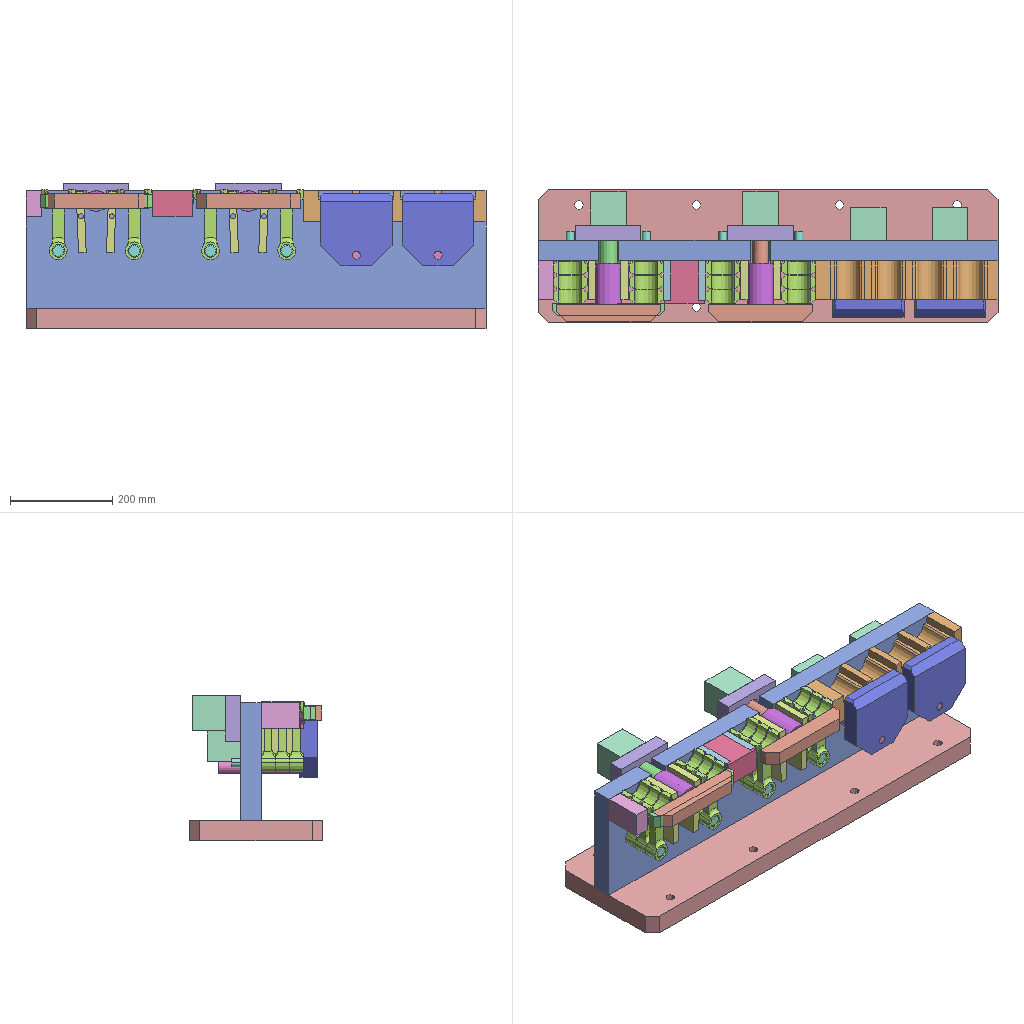Assembly | SolidWorks | 20 different items | 48 placed | box 900 x 260 x 285 mm
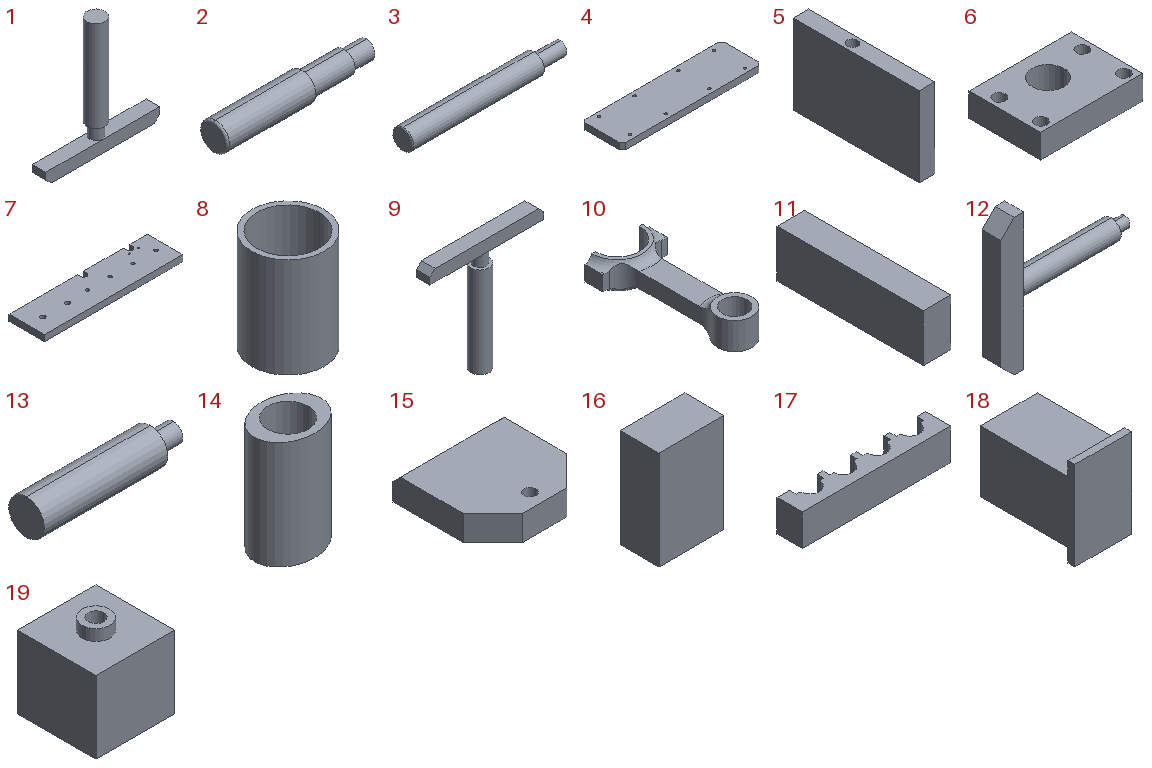Parts list (item | name | quantity | parent item | size | volume | features):
1 | (subassembly) | x1 | - | 220 x 35 x 223 mm | 309149 mm3 | features AEMSimFeature 1
2 | - | x4 | - | 138 x 25 x 25 mm | 55164 mm3 | features Fillet 1, Revolution 1
3 | - | x2 | - | 192 x 25 x 25 mm | 84936 mm3 | features Chamfer 1, Revolution 1
4 | - | x1 | - | 900 x 260 x 40 mm | 9255366 mm3 | features Chamfer 1, Extrusion 1, HoleWzd 1
5 | - | x4 | - | 15 x 120 x 76 mm | 130831 mm3 | features Extrusion 1, ICE 1
6 | - | x2 | - | 128 x 90 x 30 mm | 286695 mm3 | features Extrusion 1, HoleWzd 1, ICE 1
7 | - | x1 | - | 900 x 230 x 40 mm | 8056344 mm3 | features ICE 4, LPattern 2, Extrusion 1
8 | - | x2 | - | 29 x 29 x 40 mm | 6786 mm3 | features Extrusion 1
9 | - | x1 | in 1 | 220 x 35 x 223 mm | 309149 mm3 | features ICE 2, Chamfer 1, Extrusion 1
10 | - | x12 | - | 66 x 137 x 27.5 mm | 56707 mm3 | features Fillet 4, ICE 3, Extrusion 1, MirrorPattern 1
11 | - | x2 | - | 14.5 x 77 x 25 mm | 27913 mm3 | features Extrusion 1
12 | - | x2 | - | 199 x 30 x 204 mm | 289524 mm3 | features Chamfer 1, ICE 1, Revolution 1
13 | - | x2 | - | 125 x 30 x 30 mm | 78241 mm3 | features Revolution 1
14 | - | x2 | - | 50 x 40 x 80 mm | 69122 mm3 | features Extrusion 1, ICE 1
15 | - | x2 | - | 140 x 140 x 34 mm | 588897 mm3 | features Chamfer 3, Extrusion 1, ICE 1
16 | - | x1 | - | 50 x 30 x 76 mm | 114000 mm3 | features Extrusion 1
17 | - | x1 | - | 357 x 60 x 76 mm | 1051674 mm3 | features ICE 2, Extrusion 1, Fillet 1, LPattern 1
18 | - | x1 | - | 50 x 83 x 78 mm | 231300 mm3 | features Extrusion 1, ICE 1
19 | - | x4 | - | 70 x 70 x 75 mm | 316728 mm3 | features Extrusion 1, HoleWzd 1, ICE 1
20 | Connecting Rod02 | x1 | - | - | - | -
Mates (type | each side: item.copy, entity, surface, feature):
Coincident | 4.1 face plane Boss-Extrude1 | 7.1 face plane Boss-Extrude1 | 2 times
DistanceDim | 4.1 face plane Boss-Extrude1 | 7.1 face plane Boss-Extrude1
Coincident | 7.1 face plane Boss-Extrude1 | 16.1 face plane Boss-Extrude1 | 3 times
Coincident | 7.1 face plane Boss-Extrude1 | 10.1 face plane Boss-Extrude1
Coincident | 10.1 face plane Boss-Extrude1 | 16.1 face plane Boss-Extrude1
DistanceDim | 10.1 face plane Boss-Extrude1 | 16.1 face plane Boss-Extrude1
Concentric | 7.1 face cylinder Cut-Extrude1 | 2.1 face cylinder Revolve1
Coincident | 7.1 face plane Boss-Extrude1 | 2.1 face plane Revolve1
Coincident | 7.1 face plane Boss-Extrude1 | 17.1 face plane Boss-Extrude1 | 2 times
Coincident | 17.1 face plane Boss-Extrude1 | 10.2 face plane Boss-Extrude1
Coincident | 7.1 face plane Boss-Extrude1 | 6.1 face plane Boss-Extrude1
Concentric | 7.1 face cylinder Cut-Extrude2 | 6.1 face cylinder Cut-Extrude3
Parallel | 7.1 face plane Boss-Extrude1 | 6.1 face plane Boss-Extrude1
Concentric | 6.1 face cylinder Cut-Extrude3 | 9.1 face cylinder Boss-Extrude1
Coincident | 7.1 face plane Boss-Extrude1 | 18.1 face plane Boss-Extrude1
Coincident | 16.1 face plane Boss-Extrude1 | 18.1 face plane Boss-Extrude1
Coincident | 18.1 face plane Cut-Extrude1 | 11.1 face plane Boss-Extrude1
Coincident | 18.1 face plane Boss-Extrude1 | 11.1 face plane Boss-Extrude1 | 2 times
Coincident | 10.3 face plane Boss-Extrude1 | 11.1 face plane Boss-Extrude1
Coincident | 7.1 face plane Boss-Extrude1 | 5.1 face plane Boss-Extrude1
Concentric | 9.1 face cylinder Boss-Extrude1 | 14.1 face cylinder Cut-Extrude1
Concentric | 7.1 face cylinder Cut-Extrude4 | 5.1 face cylinder Cut-Extrude2
Coincident | 6.1 face plane Boss-Extrude1 | 19.1 face plane Boss-Extrude1
Concentric | 6.1 face cylinder Cut-Extrude3 | 19.1 face cylinder Boss-Extrude2
Coincident | 19.1 face plane Boss-Extrude2 | 12.1 face plane Revolve1
Concentric | 19.1 face cylinder M16 Tapped Hole1 | 12.1 face cylinder Revolve1
Coincident | 14.1 face plane Boss-Extrude1 | 12.1 face plane Boss-Extrude1
Coincident | 14.1 plane | 12.1 plane
Coincident | 17.1 face plane Boss-Extrude1 | 15.1 face plane Boss-Extrude1
Coincident | 12.2 face plane Boss-Extrude1 | 15.1 face plane Boss-Extrude1
Coincident | 19.2 face plane Boss-Extrude2 | 13.1 face plane Revolve1
Concentric | 19.2 face cylinder Boss-Extrude2 | 13.1 face cylinder Revolve1
Coincident | 15.1 plane | 19.2 plane
Coincident | 7.1 face plane Boss-Extrude1 | 19.2 face plane Boss-Extrude1
DistanceDim | 19.2 face plane Boss-Extrude1 | 7.1 face plane Boss-Extrude1
Coincident | 17.1 plane | 15.1 plane
Coincident | 15.1 face plane Boss-Extrude1 | 3.1 face plane Revolve1
Concentric | 15.1 face cylinder Cut-Extrude3 | 3.1 face cylinder Revolve1
Coincident | 7.1 face plane Boss-Extrude1 | 8.1 face plane Boss-Extrude1
Concentric | 7.1 face cylinder Cut-Extrude5 | 8.1 face cylinder Boss-Extrude1